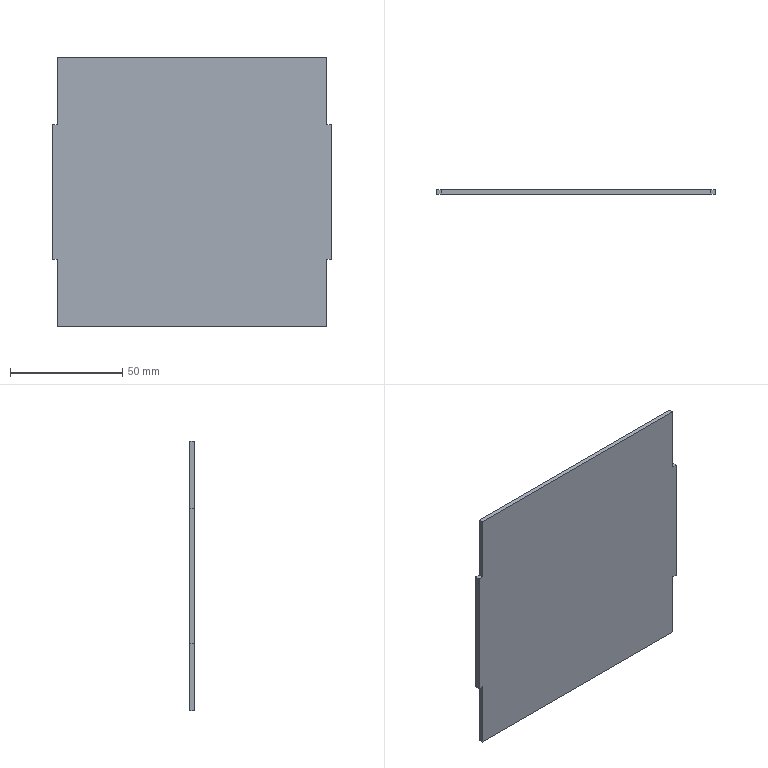Part | STEP file | JBJ-P-1003-04 | 1 solid | 14 faces | box 124 x 2 x 120 mm | volume 29280 mm3 | plane 14
STEP:
#1=CARTESIAN_POINT('',(62.,2.,30.));
#2=VERTEX_POINT('',#1);
#3=CARTESIAN_POINT('',(62.,2.,-30.));
#4=VERTEX_POINT('',#3);
#5=CARTESIAN_POINT('',(62.,2.,-60.));
#6=DIRECTION('',(0.,0.,-1.));
#7=VECTOR('',#6,1000.);
#8=LINE('',#5,#7);
#9=EDGE_CURVE('',#2,#4,#8,.T.);
#10=ORIENTED_EDGE('',*,*,#9,.F.);
#11=CARTESIAN_POINT('',(62.,0.,30.));
#12=VERTEX_POINT('',#11);
#13=CARTESIAN_POINT('',(62.,2.,30.));
#14=DIRECTION('',(0.,-1.,0.));
#15=VECTOR('',#14,1000.);
#16=LINE('',#13,#15);
#17=EDGE_CURVE('',#2,#12,#16,.T.);
#18=ORIENTED_EDGE('',*,*,#17,.T.);
#19=CARTESIAN_POINT('',(62.,0.,-30.));
#20=VERTEX_POINT('',#19);
#21=CARTESIAN_POINT('',(62.,0.,-60.));
#22=DIRECTION('',(0.,0.,-1.));
#23=VECTOR('',#22,1000.);
#24=LINE('',#21,#23);
#25=EDGE_CURVE('',#12,#20,#24,.T.);
#26=ORIENTED_EDGE('',*,*,#25,.T.);
#27=CARTESIAN_POINT('',(62.,2.,-30.));
#28=DIRECTION('',(0.,-1.,0.));
#29=VECTOR('',#28,1000.);
#30=LINE('',#27,#29);
#31=EDGE_CURVE('',#4,#20,#30,.T.);
#32=ORIENTED_EDGE('',*,*,#31,.F.);
#33=EDGE_LOOP('',(#10,#18,#26,#32));
#34=FACE_OUTER_BOUND('',#33,.T.);
#35=CARTESIAN_POINT('',(62.,2.,-60.));
#36=DIRECTION('',(-1.,0.,0.));
#37=DIRECTION('',(0.,0.,1.));
#38=AXIS2_PLACEMENT_3D('',#35,#36,#37);
#39=PLANE('',#38);
#40=ADVANCED_FACE('',(#34),#39,.F.);
#41=CARTESIAN_POINT('',(60.,0.,-60.));
#42=VERTEX_POINT('',#41);
#43=CARTESIAN_POINT('',(-60.,0.,-60.));
#44=VERTEX_POINT('',#43);
#45=CARTESIAN_POINT('',(-62.,0.,-60.));
#46=DIRECTION('',(-1.,0.,0.));
#47=VECTOR('',#46,1000.);
#48=LINE('',#45,#47);
#49=EDGE_CURVE('',#42,#44,#48,.T.);
#50=ORIENTED_EDGE('',*,*,#49,.T.);
#51=CARTESIAN_POINT('',(-60.,2.,-60.));
#52=VERTEX_POINT('',#51);
#53=CARTESIAN_POINT('',(-60.,2.,-60.));
#54=DIRECTION('',(0.,-1.,0.));
#55=VECTOR('',#54,1000.);
#56=LINE('',#53,#55);
#57=EDGE_CURVE('',#52,#44,#56,.T.);
#58=ORIENTED_EDGE('',*,*,#57,.F.);
#59=CARTESIAN_POINT('',(60.,2.,-60.));
#60=VERTEX_POINT('',#59);
#61=CARTESIAN_POINT('',(-62.,2.,-60.));
#62=DIRECTION('',(-1.,0.,0.));
#63=VECTOR('',#62,1000.);
#64=LINE('',#61,#63);
#65=EDGE_CURVE('',#60,#52,#64,.T.);
#66=ORIENTED_EDGE('',*,*,#65,.F.);
#67=CARTESIAN_POINT('',(60.,2.,-60.));
#68=DIRECTION('',(0.,-1.,0.));
#69=VECTOR('',#68,1000.);
#70=LINE('',#67,#69);
#71=EDGE_CURVE('',#60,#42,#70,.T.);
#72=ORIENTED_EDGE('',*,*,#71,.T.);
#73=EDGE_LOOP('',(#50,#58,#66,#72));
#74=FACE_OUTER_BOUND('',#73,.T.);
#75=CARTESIAN_POINT('',(-62.,2.,-60.));
#76=DIRECTION('',(0.,0.,1.));
#77=DIRECTION('',(1.,0.,0.));
#78=AXIS2_PLACEMENT_3D('',#75,#76,#77);
#79=PLANE('',#78);
#80=ADVANCED_FACE('',(#74),#79,.F.);
#81=CARTESIAN_POINT('',(-62.,2.,-30.));
#82=VERTEX_POINT('',#81);
#83=CARTESIAN_POINT('',(-62.,2.,30.));
#84=VERTEX_POINT('',#83);
#85=CARTESIAN_POINT('',(-62.,2.,-60.));
#86=DIRECTION('',(0.,0.,1.));
#87=VECTOR('',#86,1000.);
#88=LINE('',#85,#87);
#89=EDGE_CURVE('',#82,#84,#88,.T.);
#90=ORIENTED_EDGE('',*,*,#89,.F.);
#91=CARTESIAN_POINT('',(-62.,0.,-30.));
#92=VERTEX_POINT('',#91);
#93=CARTESIAN_POINT('',(-62.,2.,-30.));
#94=DIRECTION('',(0.,-1.,0.));
#95=VECTOR('',#94,1000.);
#96=LINE('',#93,#95);
#97=EDGE_CURVE('',#82,#92,#96,.T.);
#98=ORIENTED_EDGE('',*,*,#97,.T.);
#99=CARTESIAN_POINT('',(-62.,0.,30.));
#100=VERTEX_POINT('',#99);
#101=CARTESIAN_POINT('',(-62.,0.,-60.));
#102=DIRECTION('',(0.,0.,1.));
#103=VECTOR('',#102,1000.);
#104=LINE('',#101,#103);
#105=EDGE_CURVE('',#92,#100,#104,.T.);
#106=ORIENTED_EDGE('',*,*,#105,.T.);
#107=CARTESIAN_POINT('',(-62.,2.,30.));
#108=DIRECTION('',(0.,-1.,0.));
#109=VECTOR('',#108,1000.);
#110=LINE('',#107,#109);
#111=EDGE_CURVE('',#84,#100,#110,.T.);
#112=ORIENTED_EDGE('',*,*,#111,.F.);
#113=EDGE_LOOP('',(#90,#98,#106,#112));
#114=FACE_OUTER_BOUND('',#113,.T.);
#115=CARTESIAN_POINT('',(-62.,2.,-60.));
#116=DIRECTION('',(1.,0.,0.));
#117=DIRECTION('',(0.,0.,-1.));
#118=AXIS2_PLACEMENT_3D('',#115,#116,#117);
#119=PLANE('',#118);
#120=ADVANCED_FACE('',(#114),#119,.F.);
#121=CARTESIAN_POINT('',(-60.,0.,60.));
#122=VERTEX_POINT('',#121);
#123=CARTESIAN_POINT('',(60.,0.,60.));
#124=VERTEX_POINT('',#123);
#125=CARTESIAN_POINT('',(-62.,0.,60.));
#126=DIRECTION('',(1.,0.,0.));
#127=VECTOR('',#126,1000.);
#128=LINE('',#125,#127);
#129=EDGE_CURVE('',#122,#124,#128,.T.);
#130=ORIENTED_EDGE('',*,*,#129,.T.);
#131=CARTESIAN_POINT('',(60.,2.,60.));
#132=VERTEX_POINT('',#131);
#133=CARTESIAN_POINT('',(60.,2.,60.));
#134=DIRECTION('',(0.,-1.,0.));
#135=VECTOR('',#134,1000.);
#136=LINE('',#133,#135);
#137=EDGE_CURVE('',#132,#124,#136,.T.);
#138=ORIENTED_EDGE('',*,*,#137,.F.);
#139=CARTESIAN_POINT('',(-60.,2.,60.));
#140=VERTEX_POINT('',#139);
#141=CARTESIAN_POINT('',(-62.,2.,60.));
#142=DIRECTION('',(1.,0.,0.));
#143=VECTOR('',#142,1000.);
#144=LINE('',#141,#143);
#145=EDGE_CURVE('',#140,#132,#144,.T.);
#146=ORIENTED_EDGE('',*,*,#145,.F.);
#147=CARTESIAN_POINT('',(-60.,2.,60.));
#148=DIRECTION('',(0.,-1.,0.));
#149=VECTOR('',#148,1000.);
#150=LINE('',#147,#149);
#151=EDGE_CURVE('',#140,#122,#150,.T.);
#152=ORIENTED_EDGE('',*,*,#151,.T.);
#153=EDGE_LOOP('',(#130,#138,#146,#152));
#154=FACE_OUTER_BOUND('',#153,.T.);
#155=CARTESIAN_POINT('',(-62.,2.,60.));
#156=DIRECTION('',(0.,0.,-1.));
#157=DIRECTION('',(-1.,0.,0.));
#158=AXIS2_PLACEMENT_3D('',#155,#156,#157);
#159=PLANE('',#158);
#160=ADVANCED_FACE('',(#154),#159,.F.);
#161=CARTESIAN_POINT('',(60.,2.,30.));
#162=VERTEX_POINT('',#161);
#163=CARTESIAN_POINT('',(62.,2.,30.));
#164=DIRECTION('',(1.,0.,0.));
#165=VECTOR('',#164,1000.);
#166=LINE('',#163,#165);
#167=EDGE_CURVE('',#162,#2,#166,.T.);
#168=ORIENTED_EDGE('',*,*,#167,.T.);
#169=ORIENTED_EDGE('',*,*,#9,.T.);
#170=CARTESIAN_POINT('',(60.,2.,-30.));
#171=VERTEX_POINT('',#170);
#172=CARTESIAN_POINT('',(62.,2.,-30.));
#173=DIRECTION('',(-1.,0.,0.));
#174=VECTOR('',#173,1000.);
#175=LINE('',#172,#174);
#176=EDGE_CURVE('',#4,#171,#175,.T.);
#177=ORIENTED_EDGE('',*,*,#176,.T.);
#178=CARTESIAN_POINT('',(60.,2.,-60.));
#179=DIRECTION('',(0.,0.,-1.));
#180=VECTOR('',#179,1000.);
#181=LINE('',#178,#180);
#182=EDGE_CURVE('',#171,#60,#181,.T.);
#183=ORIENTED_EDGE('',*,*,#182,.T.);
#184=ORIENTED_EDGE('',*,*,#65,.T.);
#185=CARTESIAN_POINT('',(-60.,2.,-30.));
#186=VERTEX_POINT('',#185);
#187=CARTESIAN_POINT('',(-60.,2.,-60.));
#188=DIRECTION('',(0.,0.,1.));
#189=VECTOR('',#188,1000.);
#190=LINE('',#187,#189);
#191=EDGE_CURVE('',#52,#186,#190,.T.);
#192=ORIENTED_EDGE('',*,*,#191,.T.);
#193=CARTESIAN_POINT('',(-62.,2.,-30.));
#194=DIRECTION('',(-1.,0.,0.));
#195=VECTOR('',#194,1000.);
#196=LINE('',#193,#195);
#197=EDGE_CURVE('',#186,#82,#196,.T.);
#198=ORIENTED_EDGE('',*,*,#197,.T.);
#199=ORIENTED_EDGE('',*,*,#89,.T.);
#200=CARTESIAN_POINT('',(-60.,2.,30.));
#201=VERTEX_POINT('',#200);
#202=CARTESIAN_POINT('',(-62.,2.,30.));
#203=DIRECTION('',(1.,0.,0.));
#204=VECTOR('',#203,1000.);
#205=LINE('',#202,#204);
#206=EDGE_CURVE('',#84,#201,#205,.T.);
#207=ORIENTED_EDGE('',*,*,#206,.T.);
#208=CARTESIAN_POINT('',(-60.,2.,60.));
#209=DIRECTION('',(0.,0.,1.));
#210=VECTOR('',#209,1000.);
#211=LINE('',#208,#210);
#212=EDGE_CURVE('',#201,#140,#211,.T.);
#213=ORIENTED_EDGE('',*,*,#212,.T.);
#214=ORIENTED_EDGE('',*,*,#145,.T.);
#215=CARTESIAN_POINT('',(60.,2.,60.));
#216=DIRECTION('',(0.,0.,-1.));
#217=VECTOR('',#216,1000.);
#218=LINE('',#215,#217);
#219=EDGE_CURVE('',#132,#162,#218,.T.);
#220=ORIENTED_EDGE('',*,*,#219,.T.);
#221=EDGE_LOOP('',(#168,#169,#177,#183,#184,#192,#198,#199,#207,#213,#214,#220));
#222=FACE_OUTER_BOUND('',#221,.T.);
#223=CARTESIAN_POINT('',(0.,2.,0.));
#224=DIRECTION('',(0.,1.,0.));
#225=DIRECTION('',(0.,0.,1.));
#226=AXIS2_PLACEMENT_3D('',#223,#224,#225);
#227=PLANE('',#226);
#228=ADVANCED_FACE('',(#222),#227,.T.);
#229=ORIENTED_EDGE('',*,*,#25,.F.);
#230=CARTESIAN_POINT('',(60.,0.,30.));
#231=VERTEX_POINT('',#230);
#232=CARTESIAN_POINT('',(62.,0.,30.));
#233=DIRECTION('',(1.,0.,0.));
#234=VECTOR('',#233,1000.);
#235=LINE('',#232,#234);
#236=EDGE_CURVE('',#231,#12,#235,.T.);
#237=ORIENTED_EDGE('',*,*,#236,.F.);
#238=CARTESIAN_POINT('',(60.,0.,60.));
#239=DIRECTION('',(0.,0.,-1.));
#240=VECTOR('',#239,1000.);
#241=LINE('',#238,#240);
#242=EDGE_CURVE('',#124,#231,#241,.T.);
#243=ORIENTED_EDGE('',*,*,#242,.F.);
#244=ORIENTED_EDGE('',*,*,#129,.F.);
#245=CARTESIAN_POINT('',(-60.,0.,30.));
#246=VERTEX_POINT('',#245);
#247=CARTESIAN_POINT('',(-60.,0.,60.));
#248=DIRECTION('',(0.,0.,1.));
#249=VECTOR('',#248,1000.);
#250=LINE('',#247,#249);
#251=EDGE_CURVE('',#246,#122,#250,.T.);
#252=ORIENTED_EDGE('',*,*,#251,.F.);
#253=CARTESIAN_POINT('',(-62.,0.,30.));
#254=DIRECTION('',(1.,0.,0.));
#255=VECTOR('',#254,1000.);
#256=LINE('',#253,#255);
#257=EDGE_CURVE('',#100,#246,#256,.T.);
#258=ORIENTED_EDGE('',*,*,#257,.F.);
#259=ORIENTED_EDGE('',*,*,#105,.F.);
#260=CARTESIAN_POINT('',(-60.,0.,-30.));
#261=VERTEX_POINT('',#260);
#262=CARTESIAN_POINT('',(-62.,0.,-30.));
#263=DIRECTION('',(-1.,0.,0.));
#264=VECTOR('',#263,1000.);
#265=LINE('',#262,#264);
#266=EDGE_CURVE('',#261,#92,#265,.T.);
#267=ORIENTED_EDGE('',*,*,#266,.F.);
#268=CARTESIAN_POINT('',(-60.,0.,-60.));
#269=DIRECTION('',(0.,0.,1.));
#270=VECTOR('',#269,1000.);
#271=LINE('',#268,#270);
#272=EDGE_CURVE('',#44,#261,#271,.T.);
#273=ORIENTED_EDGE('',*,*,#272,.F.);
#274=ORIENTED_EDGE('',*,*,#49,.F.);
#275=CARTESIAN_POINT('',(60.,0.,-30.));
#276=VERTEX_POINT('',#275);
#277=CARTESIAN_POINT('',(60.,0.,-60.));
#278=DIRECTION('',(0.,0.,-1.));
#279=VECTOR('',#278,1000.);
#280=LINE('',#277,#279);
#281=EDGE_CURVE('',#276,#42,#280,.T.);
#282=ORIENTED_EDGE('',*,*,#281,.F.);
#283=CARTESIAN_POINT('',(62.,0.,-30.));
#284=DIRECTION('',(-1.,0.,0.));
#285=VECTOR('',#284,1000.);
#286=LINE('',#283,#285);
#287=EDGE_CURVE('',#20,#276,#286,.T.);
#288=ORIENTED_EDGE('',*,*,#287,.F.);
#289=EDGE_LOOP('',(#229,#237,#243,#244,#252,#258,#259,#267,#273,#274,#282,#288));
#290=FACE_OUTER_BOUND('',#289,.T.);
#291=CARTESIAN_POINT('',(0.,0.,0.));
#292=DIRECTION('',(0.,1.,0.));
#293=DIRECTION('',(0.,0.,1.));
#294=AXIS2_PLACEMENT_3D('',#291,#292,#293);
#295=PLANE('',#294);
#296=ADVANCED_FACE('',(#290),#295,.F.);
#297=ORIENTED_EDGE('',*,*,#281,.T.);
#298=ORIENTED_EDGE('',*,*,#71,.F.);
#299=ORIENTED_EDGE('',*,*,#182,.F.);
#300=CARTESIAN_POINT('',(60.,2.,-30.));
#301=DIRECTION('',(0.,-1.,0.));
#302=VECTOR('',#301,1000.);
#303=LINE('',#300,#302);
#304=EDGE_CURVE('',#171,#276,#303,.T.);
#305=ORIENTED_EDGE('',*,*,#304,.T.);
#306=EDGE_LOOP('',(#297,#298,#299,#305));
#307=FACE_OUTER_BOUND('',#306,.T.);
#308=CARTESIAN_POINT('',(60.,2.,-60.));
#309=DIRECTION('',(-1.,0.,0.));
#310=DIRECTION('',(0.,0.,1.));
#311=AXIS2_PLACEMENT_3D('',#308,#309,#310);
#312=PLANE('',#311);
#313=ADVANCED_FACE('',(#307),#312,.F.);
#314=ORIENTED_EDGE('',*,*,#287,.T.);
#315=ORIENTED_EDGE('',*,*,#304,.F.);
#316=ORIENTED_EDGE('',*,*,#176,.F.);
#317=ORIENTED_EDGE('',*,*,#31,.T.);
#318=EDGE_LOOP('',(#314,#315,#316,#317));
#319=FACE_OUTER_BOUND('',#318,.T.);
#320=CARTESIAN_POINT('',(62.,2.,-30.));
#321=DIRECTION('',(0.,0.,1.));
#322=DIRECTION('',(1.,0.,0.));
#323=AXIS2_PLACEMENT_3D('',#320,#321,#322);
#324=PLANE('',#323);
#325=ADVANCED_FACE('',(#319),#324,.F.);
#326=ORIENTED_EDGE('',*,*,#251,.T.);
#327=ORIENTED_EDGE('',*,*,#151,.F.);
#328=ORIENTED_EDGE('',*,*,#212,.F.);
#329=CARTESIAN_POINT('',(-60.,2.,30.));
#330=DIRECTION('',(0.,-1.,0.));
#331=VECTOR('',#330,1000.);
#332=LINE('',#329,#331);
#333=EDGE_CURVE('',#201,#246,#332,.T.);
#334=ORIENTED_EDGE('',*,*,#333,.T.);
#335=EDGE_LOOP('',(#326,#327,#328,#334));
#336=FACE_OUTER_BOUND('',#335,.T.);
#337=CARTESIAN_POINT('',(-60.,2.,60.));
#338=DIRECTION('',(1.,0.,0.));
#339=DIRECTION('',(0.,0.,-1.));
#340=AXIS2_PLACEMENT_3D('',#337,#338,#339);
#341=PLANE('',#340);
#342=ADVANCED_FACE('',(#336),#341,.F.);
#343=ORIENTED_EDGE('',*,*,#257,.T.);
#344=ORIENTED_EDGE('',*,*,#333,.F.);
#345=ORIENTED_EDGE('',*,*,#206,.F.);
#346=ORIENTED_EDGE('',*,*,#111,.T.);
#347=EDGE_LOOP('',(#343,#344,#345,#346));
#348=FACE_OUTER_BOUND('',#347,.T.);
#349=CARTESIAN_POINT('',(-62.,2.,30.));
#350=DIRECTION('',(0.,0.,-1.));
#351=DIRECTION('',(-1.,0.,0.));
#352=AXIS2_PLACEMENT_3D('',#349,#350,#351);
#353=PLANE('',#352);
#354=ADVANCED_FACE('',(#348),#353,.F.);
#355=ORIENTED_EDGE('',*,*,#266,.T.);
#356=ORIENTED_EDGE('',*,*,#97,.F.);
#357=ORIENTED_EDGE('',*,*,#197,.F.);
#358=CARTESIAN_POINT('',(-60.,2.,-30.));
#359=DIRECTION('',(0.,-1.,0.));
#360=VECTOR('',#359,1000.);
#361=LINE('',#358,#360);
#362=EDGE_CURVE('',#186,#261,#361,.T.);
#363=ORIENTED_EDGE('',*,*,#362,.T.);
#364=EDGE_LOOP('',(#355,#356,#357,#363));
#365=FACE_OUTER_BOUND('',#364,.T.);
#366=CARTESIAN_POINT('',(-62.,2.,-30.));
#367=DIRECTION('',(0.,0.,1.));
#368=DIRECTION('',(1.,0.,0.));
#369=AXIS2_PLACEMENT_3D('',#366,#367,#368);
#370=PLANE('',#369);
#371=ADVANCED_FACE('',(#365),#370,.F.);
#372=ORIENTED_EDGE('',*,*,#272,.T.);
#373=ORIENTED_EDGE('',*,*,#362,.F.);
#374=ORIENTED_EDGE('',*,*,#191,.F.);
#375=ORIENTED_EDGE('',*,*,#57,.T.);
#376=EDGE_LOOP('',(#372,#373,#374,#375));
#377=FACE_OUTER_BOUND('',#376,.T.);
#378=CARTESIAN_POINT('',(-60.,2.,-60.));
#379=DIRECTION('',(1.,0.,0.));
#380=DIRECTION('',(0.,0.,-1.));
#381=AXIS2_PLACEMENT_3D('',#378,#379,#380);
#382=PLANE('',#381);
#383=ADVANCED_FACE('',(#377),#382,.F.);
#384=ORIENTED_EDGE('',*,*,#236,.T.);
#385=ORIENTED_EDGE('',*,*,#17,.F.);
#386=ORIENTED_EDGE('',*,*,#167,.F.);
#387=CARTESIAN_POINT('',(60.,2.,30.));
#388=DIRECTION('',(0.,-1.,0.));
#389=VECTOR('',#388,1000.);
#390=LINE('',#387,#389);
#391=EDGE_CURVE('',#162,#231,#390,.T.);
#392=ORIENTED_EDGE('',*,*,#391,.T.);
#393=EDGE_LOOP('',(#384,#385,#386,#392));
#394=FACE_OUTER_BOUND('',#393,.T.);
#395=CARTESIAN_POINT('',(62.,2.,30.));
#396=DIRECTION('',(0.,0.,-1.));
#397=DIRECTION('',(-1.,0.,0.));
#398=AXIS2_PLACEMENT_3D('',#395,#396,#397);
#399=PLANE('',#398);
#400=ADVANCED_FACE('',(#394),#399,.F.);
#401=ORIENTED_EDGE('',*,*,#242,.T.);
#402=ORIENTED_EDGE('',*,*,#391,.F.);
#403=ORIENTED_EDGE('',*,*,#219,.F.);
#404=ORIENTED_EDGE('',*,*,#137,.T.);
#405=EDGE_LOOP('',(#401,#402,#403,#404));
#406=FACE_OUTER_BOUND('',#405,.T.);
#407=CARTESIAN_POINT('',(60.,2.,60.));
#408=DIRECTION('',(-1.,0.,0.));
#409=DIRECTION('',(0.,0.,1.));
#410=AXIS2_PLACEMENT_3D('',#407,#408,#409);
#411=PLANE('',#410);
#412=ADVANCED_FACE('',(#406),#411,.F.);
#413=CLOSED_SHELL('',(#40,#80,#120,#160,#228,#296,#313,#325,#342,#354,#371,#383,#400,#412));
#414=MANIFOLD_SOLID_BREP('',#413);
#415=CARTESIAN_POINT('',(0.,0.,0.));
#416=DIRECTION('',(0.,0.,1.));
#417=DIRECTION('',(1.,0.,0.));
#418=AXIS2_PLACEMENT_3D('',#415,#416,#417);
#419=(LENGTH_UNIT()NAMED_UNIT(*)SI_UNIT(.MILLI.,.METRE.));
#420=UNCERTAINTY_MEASURE_WITH_UNIT(LENGTH_MEASURE(0.00001),#419,'','');
#421=(NAMED_UNIT(*)PLANE_ANGLE_UNIT()SI_UNIT($,.RADIAN.));
#422=(NAMED_UNIT(*)SI_UNIT($,.STERADIAN.)SOLID_ANGLE_UNIT());
#423=(GEOMETRIC_REPRESENTATION_CONTEXT(3)GLOBAL_UNCERTAINTY_ASSIGNED_CONTEXT((#420))GLOBAL_UNIT_ASSIGNED_CONTEXT((#419,#421,#422))REPRESENTATION_CONTEXT('',''));
#424=ADVANCED_BREP_SHAPE_REPRESENTATION('',(#414,#418),#423);